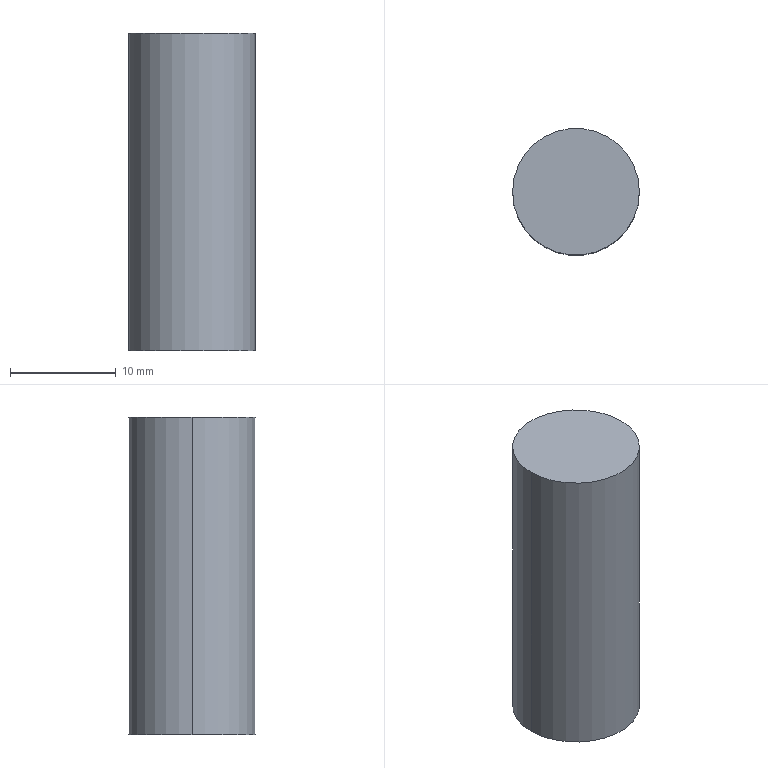Part | STEP file | MYT-A01-P31 | 1 solid | 4 faces | box 12 x 12 x 30 mm | volume 3393 mm3 | cylinder 2 | plane 2 | commonest cylinder face diameters 12 x2
STEP:
#1=CARTESIAN_POINT('',(6.,0.,30.));
#2=VERTEX_POINT('',#1);
#3=CARTESIAN_POINT('',(-6.,0.,30.));
#4=VERTEX_POINT('',#3);
#5=CARTESIAN_POINT('',(0.,0.,30.));
#6=DIRECTION('',(0.,0.,1.));
#7=DIRECTION('',(1.,0.,0.));
#8=AXIS2_PLACEMENT_3D('',#5,#6,#7);
#9=CIRCLE('',#8,6.);
#10=EDGE_CURVE('',#2,#4,#9,.T.);
#11=ORIENTED_EDGE('',*,*,#10,.F.);
#12=CARTESIAN_POINT('',(6.,0.,0.));
#13=VERTEX_POINT('',#12);
#14=CARTESIAN_POINT('',(6.,0.,30.));
#15=DIRECTION('',(0.,0.,-1.));
#16=VECTOR('',#15,1000.);
#17=LINE('',#14,#16);
#18=EDGE_CURVE('',#2,#13,#17,.T.);
#19=ORIENTED_EDGE('',*,*,#18,.T.);
#20=CARTESIAN_POINT('',(-6.,0.,0.));
#21=VERTEX_POINT('',#20);
#22=CARTESIAN_POINT('',(0.,0.,0.));
#23=DIRECTION('',(0.,0.,1.));
#24=DIRECTION('',(1.,0.,0.));
#25=AXIS2_PLACEMENT_3D('',#22,#23,#24);
#26=CIRCLE('',#25,6.);
#27=EDGE_CURVE('',#13,#21,#26,.T.);
#28=ORIENTED_EDGE('',*,*,#27,.T.);
#29=CARTESIAN_POINT('',(-6.,0.,30.));
#30=DIRECTION('',(0.,0.,-1.));
#31=VECTOR('',#30,1000.);
#32=LINE('',#29,#31);
#33=EDGE_CURVE('',#4,#21,#32,.T.);
#34=ORIENTED_EDGE('',*,*,#33,.F.);
#35=EDGE_LOOP('',(#11,#19,#28,#34));
#36=FACE_OUTER_BOUND('',#35,.T.);
#37=CARTESIAN_POINT('',(0.,0.,30.));
#38=DIRECTION('',(0.,0.,-1.));
#39=DIRECTION('',(-1.,0.,0.));
#40=AXIS2_PLACEMENT_3D('',#37,#38,#39);
#41=CYLINDRICAL_SURFACE('',#40,6.);
#42=ADVANCED_FACE('',(#36),#41,.T.);
#43=ORIENTED_EDGE('',*,*,#18,.F.);
#44=CARTESIAN_POINT('',(0.,0.,30.));
#45=DIRECTION('',(0.,0.,1.));
#46=DIRECTION('',(1.,0.,0.));
#47=AXIS2_PLACEMENT_3D('',#44,#45,#46);
#48=CIRCLE('',#47,6.);
#49=EDGE_CURVE('',#4,#2,#48,.T.);
#50=ORIENTED_EDGE('',*,*,#49,.F.);
#51=ORIENTED_EDGE('',*,*,#33,.T.);
#52=CARTESIAN_POINT('',(0.,0.,0.));
#53=DIRECTION('',(0.,0.,1.));
#54=DIRECTION('',(1.,0.,0.));
#55=AXIS2_PLACEMENT_3D('',#52,#53,#54);
#56=CIRCLE('',#55,6.);
#57=EDGE_CURVE('',#21,#13,#56,.T.);
#58=ORIENTED_EDGE('',*,*,#57,.T.);
#59=EDGE_LOOP('',(#43,#50,#51,#58));
#60=FACE_OUTER_BOUND('',#59,.T.);
#61=CARTESIAN_POINT('',(0.,0.,30.));
#62=DIRECTION('',(0.,0.,-1.));
#63=DIRECTION('',(-1.,0.,0.));
#64=AXIS2_PLACEMENT_3D('',#61,#62,#63);
#65=CYLINDRICAL_SURFACE('',#64,6.);
#66=ADVANCED_FACE('',(#60),#65,.T.);
#67=ORIENTED_EDGE('',*,*,#49,.T.);
#68=ORIENTED_EDGE('',*,*,#10,.T.);
#69=EDGE_LOOP('',(#67,#68));
#70=FACE_OUTER_BOUND('',#69,.T.);
#71=CARTESIAN_POINT('',(0.,0.,30.));
#72=DIRECTION('',(0.,0.,1.));
#73=DIRECTION('',(1.,0.,0.));
#74=AXIS2_PLACEMENT_3D('',#71,#72,#73);
#75=PLANE('',#74);
#76=ADVANCED_FACE('',(#70),#75,.T.);
#77=ORIENTED_EDGE('',*,*,#57,.F.);
#78=ORIENTED_EDGE('',*,*,#27,.F.);
#79=EDGE_LOOP('',(#77,#78));
#80=FACE_OUTER_BOUND('',#79,.T.);
#81=CARTESIAN_POINT('',(0.,0.,0.));
#82=DIRECTION('',(0.,0.,1.));
#83=DIRECTION('',(1.,0.,0.));
#84=AXIS2_PLACEMENT_3D('',#81,#82,#83);
#85=PLANE('',#84);
#86=ADVANCED_FACE('',(#80),#85,.F.);
#87=CLOSED_SHELL('',(#42,#66,#76,#86));
#88=MANIFOLD_SOLID_BREP('',#87);
#89=CARTESIAN_POINT('',(0.,0.,0.));
#90=DIRECTION('',(0.,0.,1.));
#91=DIRECTION('',(1.,0.,0.));
#92=AXIS2_PLACEMENT_3D('',#89,#90,#91);
#93=(LENGTH_UNIT()NAMED_UNIT(*)SI_UNIT(.MILLI.,.METRE.));
#94=UNCERTAINTY_MEASURE_WITH_UNIT(LENGTH_MEASURE(0.00001),#93,'','');
#95=(NAMED_UNIT(*)PLANE_ANGLE_UNIT()SI_UNIT($,.RADIAN.));
#96=(NAMED_UNIT(*)SI_UNIT($,.STERADIAN.)SOLID_ANGLE_UNIT());
#97=(GEOMETRIC_REPRESENTATION_CONTEXT(3)GLOBAL_UNCERTAINTY_ASSIGNED_CONTEXT((#94))GLOBAL_UNIT_ASSIGNED_CONTEXT((#93,#95,#96))REPRESENTATION_CONTEXT('',''));
#98=ADVANCED_BREP_SHAPE_REPRESENTATION('',(#88,#92),#97);